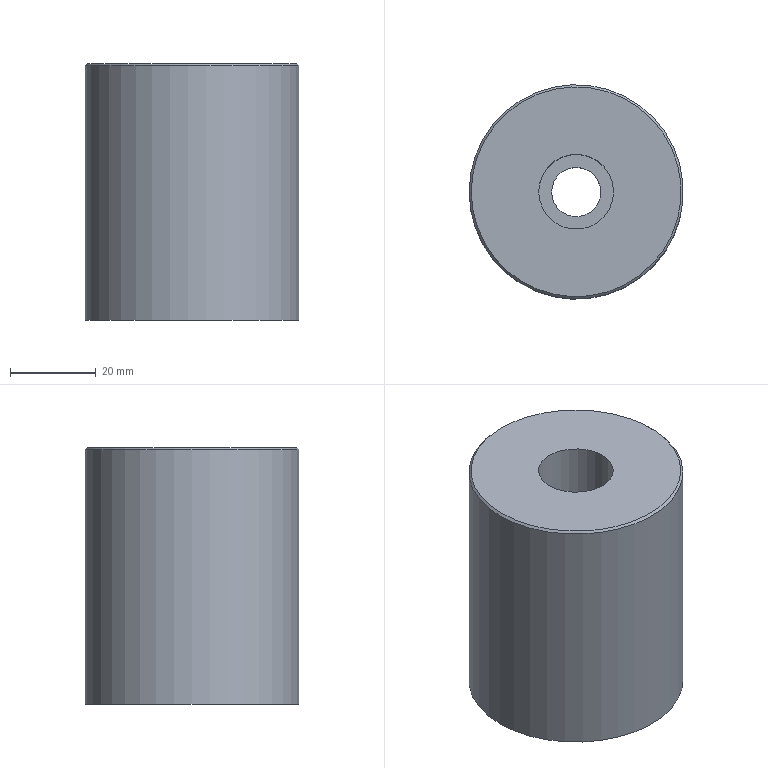Part | NX | features solid 2 | 1 solid | 7 faces | box 50 x 50 x 60 mm | volume 106092 mm3 | plane 3 | cylinder 3 | cone 1 | commonest cylinder face diameters 11.5 x1 17.5 x1 50 x1
STEP:
#1=CARTESIAN_POINT('',(335.,-370.,-90.));
#2=VERTEX_POINT('',#1);
#3=CARTESIAN_POINT('',(360.,-370.,-90.));
#4=DIRECTION('',(0.,0.,1.));
#5=DIRECTION('',(-1.,0.,0.));
#6=AXIS2_PLACEMENT_3D('',#3,#4,#5);
#7=CIRCLE('',#6,25.);
#8=EDGE_CURVE('',#2,#2,#7,.T.);
#9=ORIENTED_EDGE('',*,*,#8,.F.);
#10=EDGE_LOOP('',(#9));
#11=FACE_BOUND('',#10,.T.);
#12=CARTESIAN_POINT('',(354.25,-370.,-90.));
#13=VERTEX_POINT('',#12);
#14=CARTESIAN_POINT('',(360.,-370.,-90.));
#15=DIRECTION('',(0.,0.,1.));
#16=DIRECTION('',(-1.,0.,0.));
#17=AXIS2_PLACEMENT_3D('',#14,#15,#16);
#18=CIRCLE('',#17,5.75);
#19=EDGE_CURVE('',#13,#13,#18,.T.);
#20=ORIENTED_EDGE('',*,*,#19,.T.);
#21=EDGE_LOOP('',(#20));
#22=FACE_BOUND('',#21,.T.);
#23=CARTESIAN_POINT('',(360.,-370.,-90.));
#24=DIRECTION('',(0.,0.,1.));
#25=DIRECTION('',(-1.,0.,0.));
#26=AXIS2_PLACEMENT_3D('',#23,#24,#25);
#27=PLANE('',#26);
#28=ADVANCED_FACE('',(#11,#22),#27,.F.);
#29=CARTESIAN_POINT('',(351.25,-370.,-70.));
#30=VERTEX_POINT('',#29);
#31=CARTESIAN_POINT('',(360.,-370.,-70.));
#32=DIRECTION('',(0.,0.,1.));
#33=DIRECTION('',(-1.,0.,0.));
#34=AXIS2_PLACEMENT_3D('',#31,#32,#33);
#35=CIRCLE('',#34,8.75);
#36=EDGE_CURVE('',#30,#30,#35,.T.);
#37=ORIENTED_EDGE('',*,*,#36,.T.);
#38=EDGE_LOOP('',(#37));
#39=FACE_BOUND('',#38,.T.);
#40=CARTESIAN_POINT('',(354.25,-370.,-70.));
#41=VERTEX_POINT('',#40);
#42=CARTESIAN_POINT('',(360.,-370.,-70.));
#43=DIRECTION('',(0.,0.,1.));
#44=DIRECTION('',(-1.,0.,0.));
#45=AXIS2_PLACEMENT_3D('',#42,#43,#44);
#46=CIRCLE('',#45,5.75);
#47=EDGE_CURVE('',#41,#41,#46,.T.);
#48=ORIENTED_EDGE('',*,*,#47,.F.);
#49=EDGE_LOOP('',(#48));
#50=FACE_BOUND('',#49,.T.);
#51=CARTESIAN_POINT('',(360.,-370.,-70.));
#52=DIRECTION('',(0.,0.,1.));
#53=DIRECTION('',(-1.,0.,0.));
#54=AXIS2_PLACEMENT_3D('',#51,#52,#53);
#55=PLANE('',#54);
#56=ADVANCED_FACE('',(#39,#50),#55,.T.);
#57=CARTESIAN_POINT('',(335.5,-370.,-30.));
#58=VERTEX_POINT('',#57);
#59=CARTESIAN_POINT('',(360.,-370.,-30.));
#60=DIRECTION('',(0.,0.,1.));
#61=DIRECTION('',(-1.,0.,0.));
#62=AXIS2_PLACEMENT_3D('',#59,#60,#61);
#63=CIRCLE('',#62,24.5);
#64=EDGE_CURVE('',#58,#58,#63,.T.);
#65=ORIENTED_EDGE('',*,*,#64,.T.);
#66=EDGE_LOOP('',(#65));
#67=FACE_BOUND('',#66,.T.);
#68=CARTESIAN_POINT('',(351.25,-370.,-30.));
#69=VERTEX_POINT('',#68);
#70=CARTESIAN_POINT('',(360.,-370.,-30.));
#71=DIRECTION('',(0.,0.,1.));
#72=DIRECTION('',(-1.,0.,0.));
#73=AXIS2_PLACEMENT_3D('',#70,#71,#72);
#74=CIRCLE('',#73,8.75);
#75=EDGE_CURVE('',#69,#69,#74,.T.);
#76=ORIENTED_EDGE('',*,*,#75,.F.);
#77=EDGE_LOOP('',(#76));
#78=FACE_BOUND('',#77,.T.);
#79=CARTESIAN_POINT('',(360.,-370.,-30.));
#80=DIRECTION('',(0.,0.,1.));
#81=DIRECTION('',(-1.,0.,0.));
#82=AXIS2_PLACEMENT_3D('',#79,#80,#81);
#83=PLANE('',#82);
#84=ADVANCED_FACE('',(#67,#78),#83,.T.);
#85=CARTESIAN_POINT('',(335.,-370.,-30.5));
#86=VERTEX_POINT('',#85);
#87=CARTESIAN_POINT('',(360.,-370.,-30.5));
#88=DIRECTION('',(0.,0.,1.));
#89=DIRECTION('',(-1.,0.,0.));
#90=AXIS2_PLACEMENT_3D('',#87,#88,#89);
#91=CIRCLE('',#90,25.);
#92=EDGE_CURVE('',#86,#86,#91,.F.);
#93=ORIENTED_EDGE('',*,*,#92,.T.);
#94=EDGE_LOOP('',(#93));
#95=FACE_BOUND('',#94,.T.);
#96=ORIENTED_EDGE('',*,*,#8,.T.);
#97=EDGE_LOOP('',(#96));
#98=FACE_BOUND('',#97,.T.);
#99=CARTESIAN_POINT('',(360.,-370.,-30.));
#100=DIRECTION('',(0.,0.,-1.));
#101=DIRECTION('',(1.,0.,0.));
#102=AXIS2_PLACEMENT_3D('',#99,#100,#101);
#103=CYLINDRICAL_SURFACE('',#102,25.);
#104=ADVANCED_FACE('',(#95,#98),#103,.T.);
#105=ORIENTED_EDGE('',*,*,#75,.T.);
#106=EDGE_LOOP('',(#105));
#107=FACE_BOUND('',#106,.T.);
#108=ORIENTED_EDGE('',*,*,#36,.F.);
#109=EDGE_LOOP('',(#108));
#110=FACE_BOUND('',#109,.T.);
#111=CARTESIAN_POINT('',(360.,-370.,-30.));
#112=DIRECTION('',(0.,0.,-1.));
#113=DIRECTION('',(1.,0.,0.));
#114=AXIS2_PLACEMENT_3D('',#111,#112,#113);
#115=CYLINDRICAL_SURFACE('',#114,8.75);
#116=ADVANCED_FACE('',(#107,#110),#115,.F.);
#117=ORIENTED_EDGE('',*,*,#47,.T.);
#118=EDGE_LOOP('',(#117));
#119=FACE_BOUND('',#118,.T.);
#120=ORIENTED_EDGE('',*,*,#19,.F.);
#121=EDGE_LOOP('',(#120));
#122=FACE_BOUND('',#121,.T.);
#123=CARTESIAN_POINT('',(360.,-370.,-70.));
#124=DIRECTION('',(0.,0.,-1.));
#125=DIRECTION('',(1.,0.,0.));
#126=AXIS2_PLACEMENT_3D('',#123,#124,#125);
#127=CYLINDRICAL_SURFACE('',#126,5.75);
#128=ADVANCED_FACE('',(#119,#122),#127,.F.);
#129=ORIENTED_EDGE('',*,*,#92,.F.);
#130=EDGE_LOOP('',(#129));
#131=FACE_BOUND('',#130,.T.);
#132=ORIENTED_EDGE('',*,*,#64,.F.);
#133=EDGE_LOOP('',(#132));
#134=FACE_BOUND('',#133,.T.);
#135=CARTESIAN_POINT('',(360.,-370.,-30.));
#136=DIRECTION('',(0.,0.,-1.));
#137=DIRECTION('',(1.,0.,0.));
#138=AXIS2_PLACEMENT_3D('',#135,#136,#137);
#139=CONICAL_SURFACE('',#138,24.5,0.7854);
#140=ADVANCED_FACE('',(#131,#134),#139,.T.);
#141=CLOSED_SHELL('',(#28,#56,#84,#104,#116,#128,#140));
#142=MANIFOLD_SOLID_BREP('',#141);
#143=(LENGTH_UNIT()NAMED_UNIT(*)SI_UNIT(.MILLI.,.METRE.));
#144=UNCERTAINTY_MEASURE_WITH_UNIT(LENGTH_MEASURE(0.00001),#143,'','');
#145=(NAMED_UNIT(*)PLANE_ANGLE_UNIT()SI_UNIT($,.RADIAN.));
#146=(NAMED_UNIT(*)SI_UNIT($,.STERADIAN.)SOLID_ANGLE_UNIT());
#147=(GEOMETRIC_REPRESENTATION_CONTEXT(3)GLOBAL_UNCERTAINTY_ASSIGNED_CONTEXT((#144))GLOBAL_UNIT_ASSIGNED_CONTEXT((#143,#145,#146))REPRESENTATION_CONTEXT('',''));
#148=ADVANCED_BREP_SHAPE_REPRESENTATION('',(#142),#147);